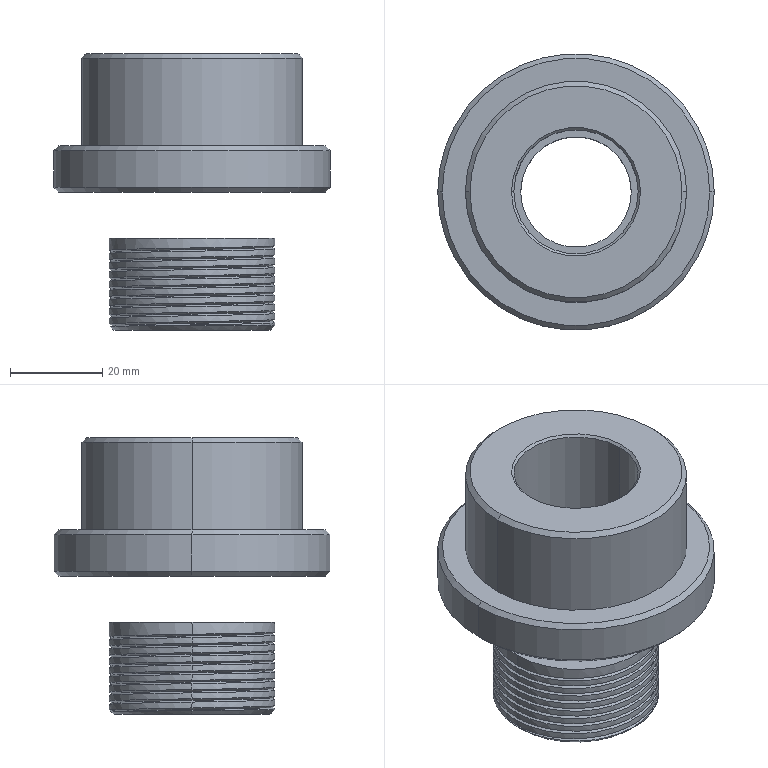Part | SolidWorks | 2 solids | 50 faces | box 60 x 60 x 60 mm | volume 59029 mm3 | cylinder 29 | cone 12 | plane 7 | spline 2 | commonest cylinder face diameters 36 x19 24 x4 27 x2 48 x2 60 x2